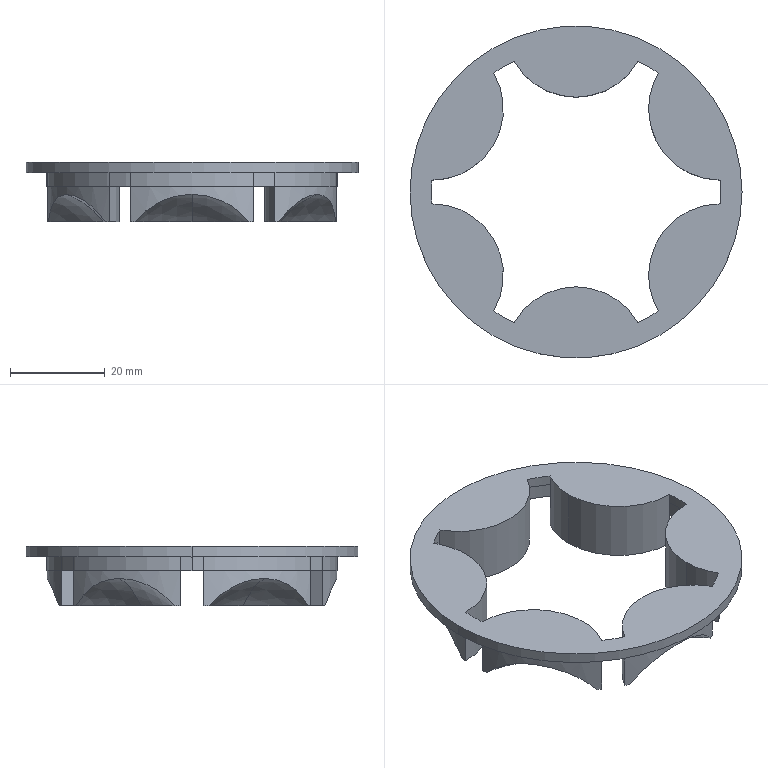Part | NX | features BREP 1 | 1 solid | 46 faces | box 70 x 70 x 12.6 mm | volume 14086 mm3 | cylinder 25 | sphere 12 | plane 9 | commonest cylinder face diameters 61 x13 30 x8 61.2 x2 70 x2